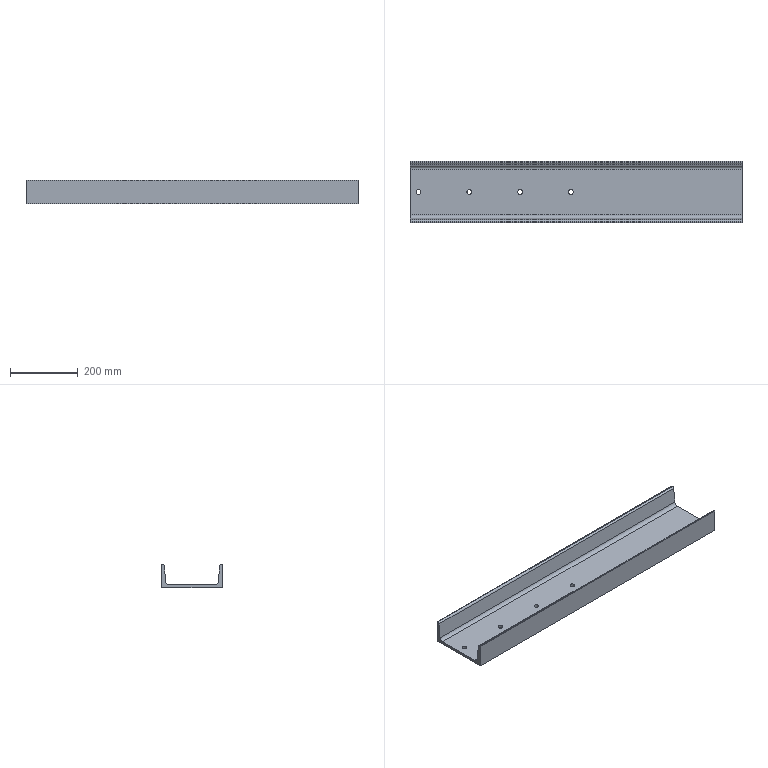Part | STEP file | 18# B Channel 980 (GB_INTERCHANGEABLE_PARTS_TM_SS 18X980)_GB_INTERCHANGEABLE_PARTS_TM_SS 18X980 | 1 solid | 22 faces | box 980 x 180 x 70 mm | volume 2864896 mm3 | cylinder 12 | plane 10 | commonest cylinder face diameters 14 x8 10.5 x2 21 x2